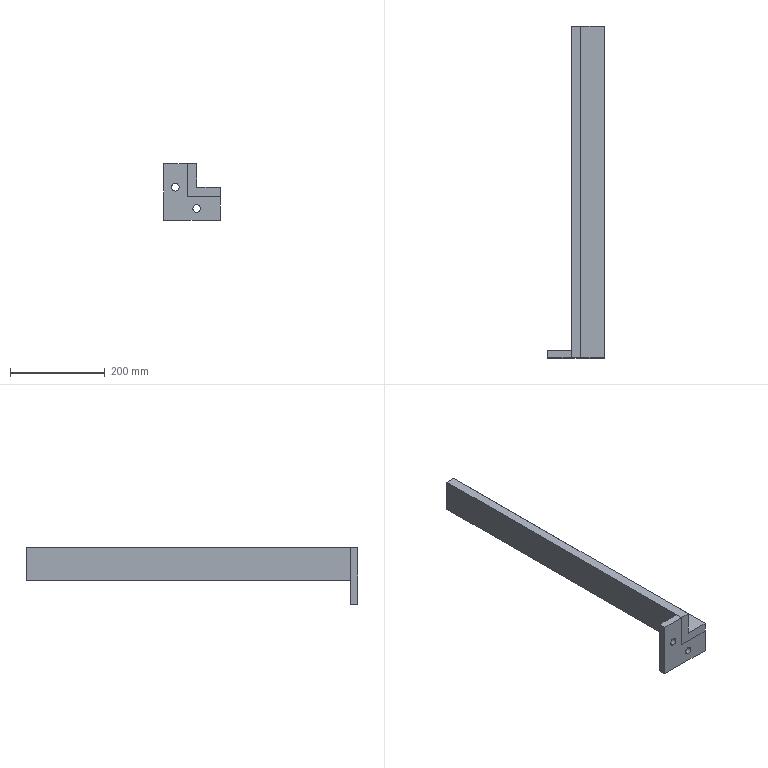Part | SolidWorks | features ICE 2, Extrusion 1 | 2 solids | 23 faces | box 120 x 700 x 120 mm | volume 1815903 mm3 | plane 17 | cylinder 6 | commonest cylinder face diameters 16 x4 6 x2
STEP:
#1=CARTESIAN_POINT('',(10.,15.,-43.));
#2=VERTEX_POINT('',#1);
#3=CARTESIAN_POINT('',(10.,15.,-27.));
#4=VERTEX_POINT('',#3);
#5=CARTESIAN_POINT('',(10.,15.,-35.));
#6=DIRECTION('',(0.,1.,0.));
#7=DIRECTION('',(0.,0.,1.));
#8=AXIS2_PLACEMENT_3D('',#5,#6,#7);
#9=CIRCLE('',#8,8.);
#10=EDGE_CURVE('',#2,#4,#9,.T.);
#11=ORIENTED_EDGE('',*,*,#10,.T.);
#12=CARTESIAN_POINT('',(10.,0.,-27.));
#13=VERTEX_POINT('',#12);
#14=CARTESIAN_POINT('',(10.,15.,-27.));
#15=DIRECTION('',(0.,-1.,0.));
#16=VECTOR('',#15,1000.);
#17=LINE('',#14,#16);
#18=EDGE_CURVE('',#4,#13,#17,.T.);
#19=ORIENTED_EDGE('',*,*,#18,.T.);
#20=CARTESIAN_POINT('',(10.,0.,-43.));
#21=VERTEX_POINT('',#20);
#22=CARTESIAN_POINT('',(10.,0.,-35.));
#23=DIRECTION('',(0.,1.,0.));
#24=DIRECTION('',(0.,0.,1.));
#25=AXIS2_PLACEMENT_3D('',#22,#23,#24);
#26=CIRCLE('',#25,8.);
#27=EDGE_CURVE('',#21,#13,#26,.T.);
#28=ORIENTED_EDGE('',*,*,#27,.F.);
#29=CARTESIAN_POINT('',(10.,15.,-43.));
#30=DIRECTION('',(0.,-1.,0.));
#31=VECTOR('',#30,1000.);
#32=LINE('',#29,#31);
#33=EDGE_CURVE('',#2,#21,#32,.T.);
#34=ORIENTED_EDGE('',*,*,#33,.F.);
#35=EDGE_LOOP('',(#11,#19,#28,#34));
#36=FACE_OUTER_BOUND('',#35,.T.);
#37=CARTESIAN_POINT('',(10.,15.,-35.));
#38=DIRECTION('',(0.,-1.,0.));
#39=DIRECTION('',(0.,0.,-1.));
#40=AXIS2_PLACEMENT_3D('',#37,#38,#39);
#41=CYLINDRICAL_SURFACE('',#40,8.);
#42=ADVANCED_FACE('',(#36),#41,.F.);
#43=CARTESIAN_POINT('',(-35.,15.,2.));
#44=VERTEX_POINT('',#43);
#45=CARTESIAN_POINT('',(-35.,15.,18.));
#46=VERTEX_POINT('',#45);
#47=CARTESIAN_POINT('',(-35.,15.,10.));
#48=DIRECTION('',(0.,1.,0.));
#49=DIRECTION('',(0.,0.,1.));
#50=AXIS2_PLACEMENT_3D('',#47,#48,#49);
#51=CIRCLE('',#50,8.);
#52=EDGE_CURVE('',#44,#46,#51,.T.);
#53=ORIENTED_EDGE('',*,*,#52,.T.);
#54=CARTESIAN_POINT('',(-35.,0.,18.));
#55=VERTEX_POINT('',#54);
#56=CARTESIAN_POINT('',(-35.,15.,18.));
#57=DIRECTION('',(0.,-1.,0.));
#58=VECTOR('',#57,1000.);
#59=LINE('',#56,#58);
#60=EDGE_CURVE('',#46,#55,#59,.T.);
#61=ORIENTED_EDGE('',*,*,#60,.T.);
#62=CARTESIAN_POINT('',(-35.,0.,2.));
#63=VERTEX_POINT('',#62);
#64=CARTESIAN_POINT('',(-35.,0.,10.));
#65=DIRECTION('',(0.,1.,0.));
#66=DIRECTION('',(0.,0.,1.));
#67=AXIS2_PLACEMENT_3D('',#64,#65,#66);
#68=CIRCLE('',#67,8.);
#69=EDGE_CURVE('',#63,#55,#68,.T.);
#70=ORIENTED_EDGE('',*,*,#69,.F.);
#71=CARTESIAN_POINT('',(-35.,15.,2.));
#72=DIRECTION('',(0.,-1.,0.));
#73=VECTOR('',#72,1000.);
#74=LINE('',#71,#73);
#75=EDGE_CURVE('',#44,#63,#74,.T.);
#76=ORIENTED_EDGE('',*,*,#75,.F.);
#77=EDGE_LOOP('',(#53,#61,#70,#76));
#78=FACE_OUTER_BOUND('',#77,.T.);
#79=CARTESIAN_POINT('',(-35.,15.,10.));
#80=DIRECTION('',(0.,-1.,0.));
#81=DIRECTION('',(0.,0.,-1.));
#82=AXIS2_PLACEMENT_3D('',#79,#80,#81);
#83=CYLINDRICAL_SURFACE('',#82,8.);
#84=ADVANCED_FACE('',(#78),#83,.F.);
#85=CARTESIAN_POINT('',(60.,15.,-10.));
#86=VERTEX_POINT('',#85);
#87=CARTESIAN_POINT('',(60.,15.,-60.));
#88=VERTEX_POINT('',#87);
#89=CARTESIAN_POINT('',(60.,15.,-10.));
#90=DIRECTION('',(0.,0.,-1.));
#91=VECTOR('',#90,1000.);
#92=LINE('',#89,#91);
#93=EDGE_CURVE('',#86,#88,#92,.T.);
#94=ORIENTED_EDGE('',*,*,#93,.T.);
#95=CARTESIAN_POINT('',(-60.,15.,-60.));
#96=VERTEX_POINT('',#95);
#97=CARTESIAN_POINT('',(-60.,15.,-60.));
#98=DIRECTION('',(-1.,0.,0.));
#99=VECTOR('',#98,1000.);
#100=LINE('',#97,#99);
#101=EDGE_CURVE('',#88,#96,#100,.T.);
#102=ORIENTED_EDGE('',*,*,#101,.T.);
#103=CARTESIAN_POINT('',(-60.,15.,60.));
#104=VERTEX_POINT('',#103);
#105=CARTESIAN_POINT('',(-60.,15.,60.));
#106=DIRECTION('',(0.,0.,1.));
#107=VECTOR('',#106,1000.);
#108=LINE('',#105,#107);
#109=EDGE_CURVE('',#96,#104,#108,.T.);
#110=ORIENTED_EDGE('',*,*,#109,.T.);
#111=CARTESIAN_POINT('',(-10.,15.,60.));
#112=VERTEX_POINT('',#111);
#113=CARTESIAN_POINT('',(-60.,15.,60.));
#114=DIRECTION('',(1.,0.,0.));
#115=VECTOR('',#114,1000.);
#116=LINE('',#113,#115);
#117=EDGE_CURVE('',#104,#112,#116,.T.);
#118=ORIENTED_EDGE('',*,*,#117,.T.);
#119=CARTESIAN_POINT('',(-10.,15.,-10.));
#120=VERTEX_POINT('',#119);
#121=CARTESIAN_POINT('',(-10.,15.,60.));
#122=DIRECTION('',(0.,0.,-1.));
#123=VECTOR('',#122,1000.);
#124=LINE('',#121,#123);
#125=EDGE_CURVE('',#112,#120,#124,.T.);
#126=ORIENTED_EDGE('',*,*,#125,.T.);
#127=CARTESIAN_POINT('',(-10.,15.,-10.));
#128=DIRECTION('',(1.,0.,0.));
#129=VECTOR('',#128,1000.);
#130=LINE('',#127,#129);
#131=EDGE_CURVE('',#120,#86,#130,.T.);
#132=ORIENTED_EDGE('',*,*,#131,.T.);
#133=EDGE_LOOP('',(#94,#102,#110,#118,#126,#132));
#134=FACE_OUTER_BOUND('',#133,.T.);
#135=ORIENTED_EDGE('',*,*,#52,.F.);
#136=CARTESIAN_POINT('',(-35.,15.,10.));
#137=DIRECTION('',(0.,1.,0.));
#138=DIRECTION('',(0.,0.,1.));
#139=AXIS2_PLACEMENT_3D('',#136,#137,#138);
#140=CIRCLE('',#139,8.);
#141=EDGE_CURVE('',#46,#44,#140,.T.);
#142=ORIENTED_EDGE('',*,*,#141,.F.);
#143=EDGE_LOOP('',(#135,#142));
#144=FACE_BOUND('',#143,.T.);
#145=ORIENTED_EDGE('',*,*,#10,.F.);
#146=CARTESIAN_POINT('',(10.,15.,-35.));
#147=DIRECTION('',(0.,1.,0.));
#148=DIRECTION('',(0.,0.,1.));
#149=AXIS2_PLACEMENT_3D('',#146,#147,#148);
#150=CIRCLE('',#149,8.);
#151=EDGE_CURVE('',#4,#2,#150,.T.);
#152=ORIENTED_EDGE('',*,*,#151,.F.);
#153=EDGE_LOOP('',(#145,#152));
#154=FACE_BOUND('',#153,.T.);
#155=CARTESIAN_POINT('',(0.,15.,0.));
#156=DIRECTION('',(0.,-1.,0.));
#157=DIRECTION('',(0.,0.,-1.));
#158=AXIS2_PLACEMENT_3D('',#155,#156,#157);
#159=PLANE('',#158);
#160=ADVANCED_FACE('',(#134,#144,#154),#159,.F.);
#161=ORIENTED_EDGE('',*,*,#69,.T.);
#162=CARTESIAN_POINT('',(-35.,0.,10.));
#163=DIRECTION('',(0.,1.,0.));
#164=DIRECTION('',(0.,0.,1.));
#165=AXIS2_PLACEMENT_3D('',#162,#163,#164);
#166=CIRCLE('',#165,8.);
#167=EDGE_CURVE('',#55,#63,#166,.T.);
#168=ORIENTED_EDGE('',*,*,#167,.T.);
#169=EDGE_LOOP('',(#161,#168));
#170=FACE_BOUND('',#169,.T.);
#171=CARTESIAN_POINT('',(60.,0.,-10.));
#172=VERTEX_POINT('',#171);
#173=CARTESIAN_POINT('',(60.,0.,-60.));
#174=VERTEX_POINT('',#173);
#175=CARTESIAN_POINT('',(60.,0.,-10.));
#176=DIRECTION('',(0.,0.,-1.));
#177=VECTOR('',#176,1000.);
#178=LINE('',#175,#177);
#179=EDGE_CURVE('',#172,#174,#178,.T.);
#180=ORIENTED_EDGE('',*,*,#179,.F.);
#181=CARTESIAN_POINT('',(-10.,0.,-10.));
#182=VERTEX_POINT('',#181);
#183=CARTESIAN_POINT('',(-10.,0.,-10.));
#184=DIRECTION('',(1.,0.,0.));
#185=VECTOR('',#184,1000.);
#186=LINE('',#183,#185);
#187=EDGE_CURVE('',#182,#172,#186,.T.);
#188=ORIENTED_EDGE('',*,*,#187,.F.);
#189=CARTESIAN_POINT('',(-10.,0.,60.));
#190=VERTEX_POINT('',#189);
#191=CARTESIAN_POINT('',(-10.,0.,60.));
#192=DIRECTION('',(0.,0.,-1.));
#193=VECTOR('',#192,1000.);
#194=LINE('',#191,#193);
#195=EDGE_CURVE('',#190,#182,#194,.T.);
#196=ORIENTED_EDGE('',*,*,#195,.F.);
#197=CARTESIAN_POINT('',(-60.,0.,60.));
#198=VERTEX_POINT('',#197);
#199=CARTESIAN_POINT('',(-60.,0.,60.));
#200=DIRECTION('',(1.,0.,0.));
#201=VECTOR('',#200,1000.);
#202=LINE('',#199,#201);
#203=EDGE_CURVE('',#198,#190,#202,.T.);
#204=ORIENTED_EDGE('',*,*,#203,.F.);
#205=CARTESIAN_POINT('',(-60.,0.,-60.));
#206=VERTEX_POINT('',#205);
#207=CARTESIAN_POINT('',(-60.,0.,60.));
#208=DIRECTION('',(0.,0.,1.));
#209=VECTOR('',#208,1000.);
#210=LINE('',#207,#209);
#211=EDGE_CURVE('',#206,#198,#210,.T.);
#212=ORIENTED_EDGE('',*,*,#211,.F.);
#213=CARTESIAN_POINT('',(-60.,0.,-60.));
#214=DIRECTION('',(-1.,0.,0.));
#215=VECTOR('',#214,1000.);
#216=LINE('',#213,#215);
#217=EDGE_CURVE('',#174,#206,#216,.T.);
#218=ORIENTED_EDGE('',*,*,#217,.F.);
#219=EDGE_LOOP('',(#180,#188,#196,#204,#212,#218));
#220=FACE_OUTER_BOUND('',#219,.T.);
#221=ORIENTED_EDGE('',*,*,#27,.T.);
#222=CARTESIAN_POINT('',(10.,0.,-35.));
#223=DIRECTION('',(0.,1.,0.));
#224=DIRECTION('',(0.,0.,1.));
#225=AXIS2_PLACEMENT_3D('',#222,#223,#224);
#226=CIRCLE('',#225,8.);
#227=EDGE_CURVE('',#13,#21,#226,.T.);
#228=ORIENTED_EDGE('',*,*,#227,.T.);
#229=EDGE_LOOP('',(#221,#228));
#230=FACE_BOUND('',#229,.T.);
#231=CARTESIAN_POINT('',(0.,0.,0.));
#232=DIRECTION('',(0.,-1.,0.));
#233=DIRECTION('',(0.,0.,-1.));
#234=AXIS2_PLACEMENT_3D('',#231,#232,#233);
#235=PLANE('',#234);
#236=ADVANCED_FACE('',(#170,#220,#230),#235,.T.);
#237=ORIENTED_EDGE('',*,*,#179,.T.);
#238=CARTESIAN_POINT('',(60.,15.,-60.));
#239=DIRECTION('',(0.,-1.,0.));
#240=VECTOR('',#239,1000.);
#241=LINE('',#238,#240);
#242=EDGE_CURVE('',#88,#174,#241,.T.);
#243=ORIENTED_EDGE('',*,*,#242,.F.);
#244=ORIENTED_EDGE('',*,*,#93,.F.);
#245=CARTESIAN_POINT('',(60.,15.,-10.));
#246=DIRECTION('',(0.,-1.,0.));
#247=VECTOR('',#246,1000.);
#248=LINE('',#245,#247);
#249=EDGE_CURVE('',#86,#172,#248,.T.);
#250=ORIENTED_EDGE('',*,*,#249,.T.);
#251=EDGE_LOOP('',(#237,#243,#244,#250));
#252=FACE_OUTER_BOUND('',#251,.T.);
#253=CARTESIAN_POINT('',(60.,15.,-10.));
#254=DIRECTION('',(-1.,0.,0.));
#255=DIRECTION('',(0.,0.,1.));
#256=AXIS2_PLACEMENT_3D('',#253,#254,#255);
#257=PLANE('',#256);
#258=ADVANCED_FACE('',(#252),#257,.F.);
#259=ORIENTED_EDGE('',*,*,#217,.T.);
#260=CARTESIAN_POINT('',(-60.,15.,-60.));
#261=DIRECTION('',(0.,-1.,0.));
#262=VECTOR('',#261,1000.);
#263=LINE('',#260,#262);
#264=EDGE_CURVE('',#96,#206,#263,.T.);
#265=ORIENTED_EDGE('',*,*,#264,.F.);
#266=ORIENTED_EDGE('',*,*,#101,.F.);
#267=ORIENTED_EDGE('',*,*,#242,.T.);
#268=EDGE_LOOP('',(#259,#265,#266,#267));
#269=FACE_OUTER_BOUND('',#268,.T.);
#270=CARTESIAN_POINT('',(-60.,15.,-60.));
#271=DIRECTION('',(0.,0.,1.));
#272=DIRECTION('',(1.,0.,0.));
#273=AXIS2_PLACEMENT_3D('',#270,#271,#272);
#274=PLANE('',#273);
#275=ADVANCED_FACE('',(#269),#274,.F.);
#276=ORIENTED_EDGE('',*,*,#211,.T.);
#277=CARTESIAN_POINT('',(-60.,15.,60.));
#278=DIRECTION('',(0.,-1.,0.));
#279=VECTOR('',#278,1000.);
#280=LINE('',#277,#279);
#281=EDGE_CURVE('',#104,#198,#280,.T.);
#282=ORIENTED_EDGE('',*,*,#281,.F.);
#283=ORIENTED_EDGE('',*,*,#109,.F.);
#284=ORIENTED_EDGE('',*,*,#264,.T.);
#285=EDGE_LOOP('',(#276,#282,#283,#284));
#286=FACE_OUTER_BOUND('',#285,.T.);
#287=CARTESIAN_POINT('',(-60.,15.,60.));
#288=DIRECTION('',(1.,0.,0.));
#289=DIRECTION('',(0.,0.,-1.));
#290=AXIS2_PLACEMENT_3D('',#287,#288,#289);
#291=PLANE('',#290);
#292=ADVANCED_FACE('',(#286),#291,.F.);
#293=ORIENTED_EDGE('',*,*,#203,.T.);
#294=CARTESIAN_POINT('',(-10.,15.,60.));
#295=DIRECTION('',(0.,-1.,0.));
#296=VECTOR('',#295,1000.);
#297=LINE('',#294,#296);
#298=EDGE_CURVE('',#112,#190,#297,.T.);
#299=ORIENTED_EDGE('',*,*,#298,.F.);
#300=ORIENTED_EDGE('',*,*,#117,.F.);
#301=ORIENTED_EDGE('',*,*,#281,.T.);
#302=EDGE_LOOP('',(#293,#299,#300,#301));
#303=FACE_OUTER_BOUND('',#302,.T.);
#304=CARTESIAN_POINT('',(-60.,15.,60.));
#305=DIRECTION('',(0.,0.,-1.));
#306=DIRECTION('',(-1.,0.,0.));
#307=AXIS2_PLACEMENT_3D('',#304,#305,#306);
#308=PLANE('',#307);
#309=ADVANCED_FACE('',(#303),#308,.F.);
#310=ORIENTED_EDGE('',*,*,#195,.T.);
#311=CARTESIAN_POINT('',(-10.,15.,-10.));
#312=DIRECTION('',(0.,-1.,0.));
#313=VECTOR('',#312,1000.);
#314=LINE('',#311,#313);
#315=EDGE_CURVE('',#120,#182,#314,.T.);
#316=ORIENTED_EDGE('',*,*,#315,.F.);
#317=ORIENTED_EDGE('',*,*,#125,.F.);
#318=ORIENTED_EDGE('',*,*,#298,.T.);
#319=EDGE_LOOP('',(#310,#316,#317,#318));
#320=FACE_OUTER_BOUND('',#319,.T.);
#321=CARTESIAN_POINT('',(-10.,15.,60.));
#322=DIRECTION('',(-1.,0.,0.));
#323=DIRECTION('',(0.,0.,1.));
#324=AXIS2_PLACEMENT_3D('',#321,#322,#323);
#325=PLANE('',#324);
#326=ADVANCED_FACE('',(#320),#325,.F.);
#327=ORIENTED_EDGE('',*,*,#187,.T.);
#328=ORIENTED_EDGE('',*,*,#249,.F.);
#329=ORIENTED_EDGE('',*,*,#131,.F.);
#330=ORIENTED_EDGE('',*,*,#315,.T.);
#331=EDGE_LOOP('',(#327,#328,#329,#330));
#332=FACE_OUTER_BOUND('',#331,.T.);
#333=CARTESIAN_POINT('',(-10.,15.,-10.));
#334=DIRECTION('',(0.,0.,-1.));
#335=DIRECTION('',(-1.,0.,0.));
#336=AXIS2_PLACEMENT_3D('',#333,#334,#335);
#337=PLANE('',#336);
#338=ADVANCED_FACE('',(#332),#337,.F.);
#339=ORIENTED_EDGE('',*,*,#60,.F.);
#340=ORIENTED_EDGE('',*,*,#141,.T.);
#341=ORIENTED_EDGE('',*,*,#75,.T.);
#342=ORIENTED_EDGE('',*,*,#167,.F.);
#343=EDGE_LOOP('',(#339,#340,#341,#342));
#344=FACE_OUTER_BOUND('',#343,.T.);
#345=CARTESIAN_POINT('',(-35.,15.,10.));
#346=DIRECTION('',(0.,-1.,0.));
#347=DIRECTION('',(0.,0.,-1.));
#348=AXIS2_PLACEMENT_3D('',#345,#346,#347);
#349=CYLINDRICAL_SURFACE('',#348,8.);
#350=ADVANCED_FACE('',(#344),#349,.F.);
#351=ORIENTED_EDGE('',*,*,#18,.F.);
#352=ORIENTED_EDGE('',*,*,#151,.T.);
#353=ORIENTED_EDGE('',*,*,#33,.T.);
#354=ORIENTED_EDGE('',*,*,#227,.F.);
#355=EDGE_LOOP('',(#351,#352,#353,#354));
#356=FACE_OUTER_BOUND('',#355,.T.);
#357=CARTESIAN_POINT('',(10.,15.,-35.));
#358=DIRECTION('',(0.,-1.,0.));
#359=DIRECTION('',(0.,0.,-1.));
#360=AXIS2_PLACEMENT_3D('',#357,#358,#359);
#361=CYLINDRICAL_SURFACE('',#360,8.);
#362=ADVANCED_FACE('',(#356),#361,.F.);
#363=CLOSED_SHELL('',(#42,#84,#160,#236,#258,#275,#292,#309,#326,#338,#350,#362));
#364=MANIFOLD_SOLID_BREP('',#363);
#365=CARTESIAN_POINT('',(0.,680.,-3.));
#366=VERTEX_POINT('',#365);
#367=CARTESIAN_POINT('',(0.,680.,3.));
#368=VERTEX_POINT('',#367);
#369=CARTESIAN_POINT('',(0.,680.,0.));
#370=DIRECTION('',(0.,1.,0.));
#371=DIRECTION('',(0.,0.,1.));
#372=AXIS2_PLACEMENT_3D('',#369,#370,#371);
#373=CIRCLE('',#372,3.);
#374=EDGE_CURVE('',#366,#368,#373,.T.);
#375=ORIENTED_EDGE('',*,*,#374,.F.);
#376=CARTESIAN_POINT('',(0.,700.,-3.));
#377=VERTEX_POINT('',#376);
#378=CARTESIAN_POINT('',(0.,680.,-3.));
#379=DIRECTION('',(0.,1.,0.));
#380=VECTOR('',#379,1000.);
#381=LINE('',#378,#380);
#382=EDGE_CURVE('',#366,#377,#381,.T.);
#383=ORIENTED_EDGE('',*,*,#382,.T.);
#384=CARTESIAN_POINT('',(0.,700.,3.));
#385=VERTEX_POINT('',#384);
#386=CARTESIAN_POINT('',(0.,700.,0.));
#387=DIRECTION('',(0.,1.,0.));
#388=DIRECTION('',(0.,0.,1.));
#389=AXIS2_PLACEMENT_3D('',#386,#387,#388);
#390=CIRCLE('',#389,3.);
#391=EDGE_CURVE('',#377,#385,#390,.T.);
#392=ORIENTED_EDGE('',*,*,#391,.T.);
#393=CARTESIAN_POINT('',(0.,680.,3.));
#394=DIRECTION('',(0.,1.,0.));
#395=VECTOR('',#394,1000.);
#396=LINE('',#393,#395);
#397=EDGE_CURVE('',#368,#385,#396,.T.);
#398=ORIENTED_EDGE('',*,*,#397,.F.);
#399=EDGE_LOOP('',(#375,#383,#392,#398));
#400=FACE_OUTER_BOUND('',#399,.T.);
#401=CARTESIAN_POINT('',(0.,680.,0.));
#402=DIRECTION('',(0.,1.,0.));
#403=DIRECTION('',(0.,0.,1.));
#404=AXIS2_PLACEMENT_3D('',#401,#402,#403);
#405=CYLINDRICAL_SURFACE('',#404,3.);
#406=ADVANCED_FACE('',(#400),#405,.F.);
#407=CARTESIAN_POINT('',(-10.,700.,60.));
#408=VERTEX_POINT('',#407);
#409=CARTESIAN_POINT('',(-10.,0.,60.));
#410=VERTEX_POINT('',#409);
#411=CARTESIAN_POINT('',(-10.,700.,60.));
#412=DIRECTION('',(0.,-1.,0.));
#413=VECTOR('',#412,1000.);
#414=LINE('',#411,#413);
#415=EDGE_CURVE('',#408,#410,#414,.T.);
#416=ORIENTED_EDGE('',*,*,#415,.T.);
#417=CARTESIAN_POINT('',(10.,0.,60.));
#418=VERTEX_POINT('',#417);
#419=CARTESIAN_POINT('',(-10.,0.,60.));
#420=DIRECTION('',(1.,0.,0.));
#421=VECTOR('',#420,1000.);
#422=LINE('',#419,#421);
#423=EDGE_CURVE('',#410,#418,#422,.T.);
#424=ORIENTED_EDGE('',*,*,#423,.T.);
#425=CARTESIAN_POINT('',(10.,700.,60.));
#426=VERTEX_POINT('',#425);
#427=CARTESIAN_POINT('',(10.,700.,60.));
#428=DIRECTION('',(0.,-1.,0.));
#429=VECTOR('',#428,1000.);
#430=LINE('',#427,#429);
#431=EDGE_CURVE('',#426,#418,#430,.T.);
#432=ORIENTED_EDGE('',*,*,#431,.F.);
#433=CARTESIAN_POINT('',(-10.,700.,60.));
#434=DIRECTION('',(1.,0.,0.));
#435=VECTOR('',#434,1000.);
#436=LINE('',#433,#435);
#437=EDGE_CURVE('',#408,#426,#436,.T.);
#438=ORIENTED_EDGE('',*,*,#437,.F.);
#439=EDGE_LOOP('',(#416,#424,#432,#438));
#440=FACE_OUTER_BOUND('',#439,.T.);
#441=CARTESIAN_POINT('',(-10.,700.,60.));
#442=DIRECTION('',(0.,0.,-1.));
#443=DIRECTION('',(-1.,0.,0.));
#444=AXIS2_PLACEMENT_3D('',#441,#442,#443);
#445=PLANE('',#444);
#446=ADVANCED_FACE('',(#440),#445,.F.);
#447=ORIENTED_EDGE('',*,*,#431,.T.);
#448=CARTESIAN_POINT('',(10.,0.,10.));
#449=VERTEX_POINT('',#448);
#450=CARTESIAN_POINT('',(10.,0.,60.));
#451=DIRECTION('',(0.,0.,-1.));
#452=VECTOR('',#451,1000.);
#453=LINE('',#450,#452);
#454=EDGE_CURVE('',#418,#449,#453,.T.);
#455=ORIENTED_EDGE('',*,*,#454,.T.);
#456=CARTESIAN_POINT('',(10.,700.,10.));
#457=VERTEX_POINT('',#456);
#458=CARTESIAN_POINT('',(10.,700.,10.));
#459=DIRECTION('',(0.,-1.,0.));
#460=VECTOR('',#459,1000.);
#461=LINE('',#458,#460);
#462=EDGE_CURVE('',#457,#449,#461,.T.);
#463=ORIENTED_EDGE('',*,*,#462,.F.);
#464=CARTESIAN_POINT('',(10.,700.,60.));
#465=DIRECTION('',(0.,0.,-1.));
#466=VECTOR('',#465,1000.);
#467=LINE('',#464,#466);
#468=EDGE_CURVE('',#426,#457,#467,.T.);
#469=ORIENTED_EDGE('',*,*,#468,.F.);
#470=EDGE_LOOP('',(#447,#455,#463,#469));
#471=FACE_OUTER_BOUND('',#470,.T.);
#472=CARTESIAN_POINT('',(10.,700.,60.));
#473=DIRECTION('',(-1.,0.,0.));
#474=DIRECTION('',(0.,0.,1.));
#475=AXIS2_PLACEMENT_3D('',#472,#473,#474);
#476=PLANE('',#475);
#477=ADVANCED_FACE('',(#471),#476,.F.);
#478=ORIENTED_EDGE('',*,*,#462,.T.);
#479=CARTESIAN_POINT('',(60.,0.,10.));
#480=VERTEX_POINT('',#479);
#481=CARTESIAN_POINT('',(10.,0.,10.));
#482=DIRECTION('',(1.,0.,0.));
#483=VECTOR('',#482,1000.);
#484=LINE('',#481,#483);
#485=EDGE_CURVE('',#449,#480,#484,.T.);
#486=ORIENTED_EDGE('',*,*,#485,.T.);
#487=CARTESIAN_POINT('',(60.,700.,10.));
#488=VERTEX_POINT('',#487);
#489=CARTESIAN_POINT('',(60.,700.,10.));
#490=DIRECTION('',(0.,-1.,0.));
#491=VECTOR('',#490,1000.);
#492=LINE('',#489,#491);
#493=EDGE_CURVE('',#488,#480,#492,.T.);
#494=ORIENTED_EDGE('',*,*,#493,.F.);
#495=CARTESIAN_POINT('',(10.,700.,10.));
#496=DIRECTION('',(1.,0.,0.));
#497=VECTOR('',#496,1000.);
#498=LINE('',#495,#497);
#499=EDGE_CURVE('',#457,#488,#498,.T.);
#500=ORIENTED_EDGE('',*,*,#499,.F.);
#501=EDGE_LOOP('',(#478,#486,#494,#500));
#502=FACE_OUTER_BOUND('',#501,.T.);
#503=CARTESIAN_POINT('',(10.,700.,10.));
#504=DIRECTION('',(0.,0.,-1.));
#505=DIRECTION('',(-1.,0.,0.));
#506=AXIS2_PLACEMENT_3D('',#503,#504,#505);
#507=PLANE('',#506);
#508=ADVANCED_FACE('',(#502),#507,.F.);
#509=ORIENTED_EDGE('',*,*,#493,.T.);
#510=CARTESIAN_POINT('',(60.,0.,-10.));
#511=VERTEX_POINT('',#510);
#512=CARTESIAN_POINT('',(60.,0.,-10.));
#513=DIRECTION('',(0.,0.,-1.));
#514=VECTOR('',#513,1000.);
#515=LINE('',#512,#514);
#516=EDGE_CURVE('',#480,#511,#515,.T.);
#517=ORIENTED_EDGE('',*,*,#516,.T.);
#518=CARTESIAN_POINT('',(60.,700.,-10.));
#519=VERTEX_POINT('',#518);
#520=CARTESIAN_POINT('',(60.,700.,-10.));
#521=DIRECTION('',(0.,-1.,0.));
#522=VECTOR('',#521,1000.);
#523=LINE('',#520,#522);
#524=EDGE_CURVE('',#519,#511,#523,.T.);
#525=ORIENTED_EDGE('',*,*,#524,.F.);
#526=CARTESIAN_POINT('',(60.,700.,-10.));
#527=DIRECTION('',(0.,0.,-1.));
#528=VECTOR('',#527,1000.);
#529=LINE('',#526,#528);
#530=EDGE_CURVE('',#488,#519,#529,.T.);
#531=ORIENTED_EDGE('',*,*,#530,.F.);
#532=EDGE_LOOP('',(#509,#517,#525,#531));
#533=FACE_OUTER_BOUND('',#532,.T.);
#534=CARTESIAN_POINT('',(60.,700.,-10.));
#535=DIRECTION('',(-1.,0.,0.));
#536=DIRECTION('',(0.,0.,1.));
#537=AXIS2_PLACEMENT_3D('',#534,#535,#536);
#538=PLANE('',#537);
#539=ADVANCED_FACE('',(#533),#538,.F.);
#540=ORIENTED_EDGE('',*,*,#524,.T.);
#541=CARTESIAN_POINT('',(-10.,0.,-10.));
#542=VERTEX_POINT('',#541);
#543=CARTESIAN_POINT('',(-10.,0.,-10.));
#544=DIRECTION('',(-1.,0.,0.));
#545=VECTOR('',#544,1000.);
#546=LINE('',#543,#545);
#547=EDGE_CURVE('',#511,#542,#546,.T.);
#548=ORIENTED_EDGE('',*,*,#547,.T.);
#549=CARTESIAN_POINT('',(-10.,700.,-10.));
#550=VERTEX_POINT('',#549);
#551=CARTESIAN_POINT('',(-10.,700.,-10.));
#552=DIRECTION('',(0.,-1.,0.));
#553=VECTOR('',#552,1000.);
#554=LINE('',#551,#553);
#555=EDGE_CURVE('',#550,#542,#554,.T.);
#556=ORIENTED_EDGE('',*,*,#555,.F.);
#557=CARTESIAN_POINT('',(-10.,700.,-10.));
#558=DIRECTION('',(-1.,0.,0.));
#559=VECTOR('',#558,1000.);
#560=LINE('',#557,#559);
#561=EDGE_CURVE('',#519,#550,#560,.T.);
#562=ORIENTED_EDGE('',*,*,#561,.F.);
#563=EDGE_LOOP('',(#540,#548,#556,#562));
#564=FACE_OUTER_BOUND('',#563,.T.);
#565=CARTESIAN_POINT('',(-10.,700.,-10.));
#566=DIRECTION('',(0.,0.,1.));
#567=DIRECTION('',(1.,0.,0.));
#568=AXIS2_PLACEMENT_3D('',#565,#566,#567);
#569=PLANE('',#568);
#570=ADVANCED_FACE('',(#564),#569,.F.);
#571=ORIENTED_EDGE('',*,*,#555,.T.);
#572=CARTESIAN_POINT('',(-10.,0.,60.));
#573=DIRECTION('',(0.,0.,1.));
#574=VECTOR('',#573,1000.);
#575=LINE('',#572,#574);
#576=EDGE_CURVE('',#542,#410,#575,.T.);
#577=ORIENTED_EDGE('',*,*,#576,.T.);
#578=ORIENTED_EDGE('',*,*,#415,.F.);
#579=CARTESIAN_POINT('',(-10.,700.,60.));
#580=DIRECTION('',(0.,0.,1.));
#581=VECTOR('',#580,1000.);
#582=LINE('',#579,#581);
#583=EDGE_CURVE('',#550,#408,#582,.T.);
#584=ORIENTED_EDGE('',*,*,#583,.F.);
#585=EDGE_LOOP('',(#571,#577,#578,#584));
#586=FACE_OUTER_BOUND('',#585,.T.);
#587=CARTESIAN_POINT('',(-10.,700.,60.));
#588=DIRECTION('',(1.,0.,0.));
#589=DIRECTION('',(0.,0.,-1.));
#590=AXIS2_PLACEMENT_3D('',#587,#588,#589);
#591=PLANE('',#590);
#592=ADVANCED_FACE('',(#586),#591,.F.);
#593=CARTESIAN_POINT('',(0.,700.,0.));
#594=DIRECTION('',(0.,1.,0.));
#595=DIRECTION('',(0.,0.,1.));
#596=AXIS2_PLACEMENT_3D('',#593,#594,#595);
#597=CIRCLE('',#596,3.);
#598=EDGE_CURVE('',#385,#377,#597,.T.);
#599=ORIENTED_EDGE('',*,*,#598,.F.);
#600=ORIENTED_EDGE('',*,*,#391,.F.);
#601=EDGE_LOOP('',(#599,#600));
#602=FACE_BOUND('',#601,.T.);
#603=ORIENTED_EDGE('',*,*,#437,.T.);
#604=ORIENTED_EDGE('',*,*,#468,.T.);
#605=ORIENTED_EDGE('',*,*,#499,.T.);
#606=ORIENTED_EDGE('',*,*,#530,.T.);
#607=ORIENTED_EDGE('',*,*,#561,.T.);
#608=ORIENTED_EDGE('',*,*,#583,.T.);
#609=EDGE_LOOP('',(#603,#604,#605,#606,#607,#608));
#610=FACE_OUTER_BOUND('',#609,.T.);
#611=CARTESIAN_POINT('',(0.,700.,0.));
#612=DIRECTION('',(0.,1.,0.));
#613=DIRECTION('',(0.,0.,1.));
#614=AXIS2_PLACEMENT_3D('',#611,#612,#613);
#615=PLANE('',#614);
#616=ADVANCED_FACE('',(#602,#610),#615,.T.);
#617=ORIENTED_EDGE('',*,*,#423,.F.);
#618=ORIENTED_EDGE('',*,*,#576,.F.);
#619=ORIENTED_EDGE('',*,*,#547,.F.);
#620=ORIENTED_EDGE('',*,*,#516,.F.);
#621=ORIENTED_EDGE('',*,*,#485,.F.);
#622=ORIENTED_EDGE('',*,*,#454,.F.);
#623=EDGE_LOOP('',(#617,#618,#619,#620,#621,#622));
#624=FACE_OUTER_BOUND('',#623,.T.);
#625=CARTESIAN_POINT('',(0.,0.,0.));
#626=DIRECTION('',(0.,1.,0.));
#627=DIRECTION('',(0.,0.,1.));
#628=AXIS2_PLACEMENT_3D('',#625,#626,#627);
#629=PLANE('',#628);
#630=ADVANCED_FACE('',(#624),#629,.F.);
#631=ORIENTED_EDGE('',*,*,#382,.F.);
#632=CARTESIAN_POINT('',(0.,680.,0.));
#633=DIRECTION('',(0.,1.,0.));
#634=DIRECTION('',(0.,0.,1.));
#635=AXIS2_PLACEMENT_3D('',#632,#633,#634);
#636=CIRCLE('',#635,3.);
#637=EDGE_CURVE('',#368,#366,#636,.T.);
#638=ORIENTED_EDGE('',*,*,#637,.F.);
#639=ORIENTED_EDGE('',*,*,#397,.T.);
#640=ORIENTED_EDGE('',*,*,#598,.T.);
#641=EDGE_LOOP('',(#631,#638,#639,#640));
#642=FACE_OUTER_BOUND('',#641,.T.);
#643=CARTESIAN_POINT('',(0.,680.,0.));
#644=DIRECTION('',(0.,1.,0.));
#645=DIRECTION('',(0.,0.,1.));
#646=AXIS2_PLACEMENT_3D('',#643,#644,#645);
#647=CYLINDRICAL_SURFACE('',#646,3.);
#648=ADVANCED_FACE('',(#642),#647,.F.);
#649=ORIENTED_EDGE('',*,*,#637,.T.);
#650=ORIENTED_EDGE('',*,*,#374,.T.);
#651=EDGE_LOOP('',(#649,#650));
#652=FACE_OUTER_BOUND('',#651,.T.);
#653=CARTESIAN_POINT('',(0.,680.,0.));
#654=DIRECTION('',(0.,1.,0.));
#655=DIRECTION('',(0.,0.,1.));
#656=AXIS2_PLACEMENT_3D('',#653,#654,#655);
#657=PLANE('',#656);
#658=ADVANCED_FACE('',(#652),#657,.T.);
#659=CLOSED_SHELL('',(#406,#446,#477,#508,#539,#570,#592,#616,#630,#648,#658));
#660=MANIFOLD_SOLID_BREP('',#659);
#661=CARTESIAN_POINT('',(0.,0.,0.));
#662=DIRECTION('',(0.,0.,1.));
#663=DIRECTION('',(1.,0.,0.));
#664=AXIS2_PLACEMENT_3D('',#661,#662,#663);
#665=(LENGTH_UNIT()NAMED_UNIT(*)SI_UNIT(.MILLI.,.METRE.));
#666=UNCERTAINTY_MEASURE_WITH_UNIT(LENGTH_MEASURE(0.00001),#665,'','');
#667=(NAMED_UNIT(*)PLANE_ANGLE_UNIT()SI_UNIT($,.RADIAN.));
#668=(NAMED_UNIT(*)SI_UNIT($,.STERADIAN.)SOLID_ANGLE_UNIT());
#669=(GEOMETRIC_REPRESENTATION_CONTEXT(3)GLOBAL_UNCERTAINTY_ASSIGNED_CONTEXT((#666))GLOBAL_UNIT_ASSIGNED_CONTEXT((#665,#667,#668))REPRESENTATION_CONTEXT('',''));
#670=ADVANCED_BREP_SHAPE_REPRESENTATION('',(#364,#660,#664),#669);